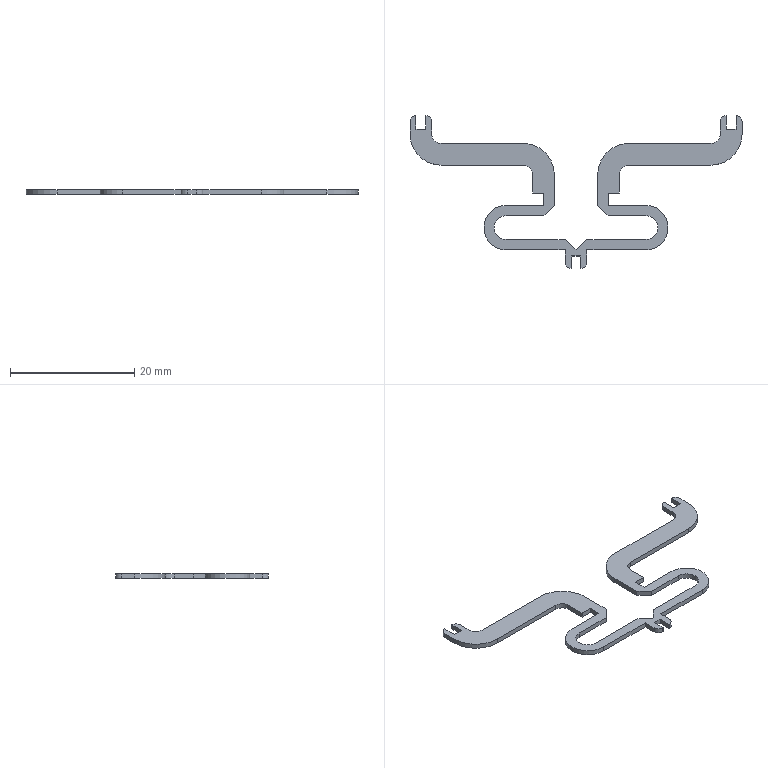Part | STEP file | 2-in-1 splitter plate | 1 solid | 61 faces | box 53.51 x 24.649 x 0.8 mm | volume 239.301 mm3 | plane 43 | cylinder 18 | commonest cylinder face diameters 2 x6 2.98 x4 10 x4 3.84 x2 7.16 x2